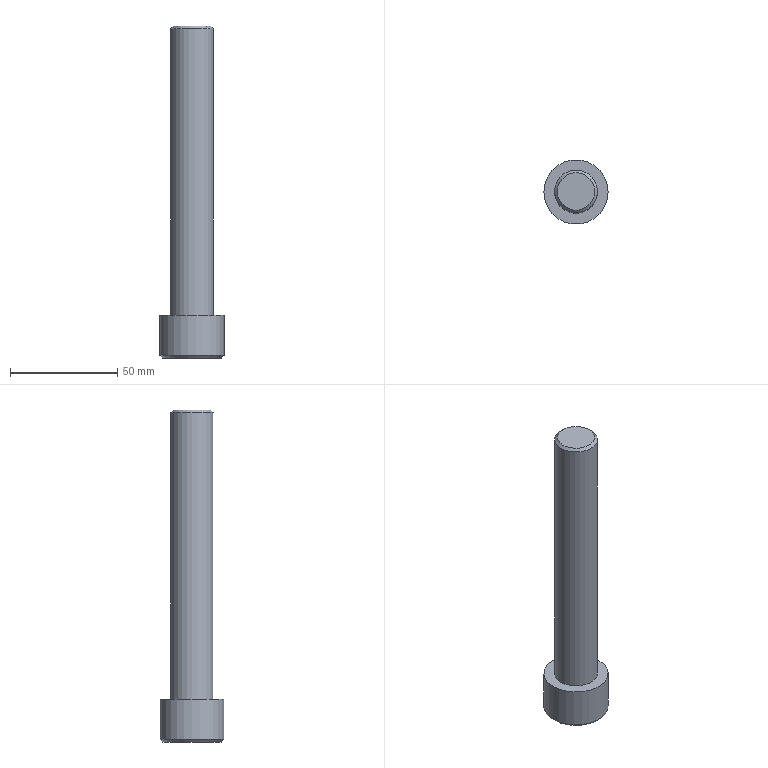Part | STEP file | solid 79 | 1 solid | 14 faces | box 30 x 30 x 155 mm | volume 53677 mm3 | plane 10 | cone 2 | cylinder 2 | commonest cylinder face diameters 20 x1 30 x1